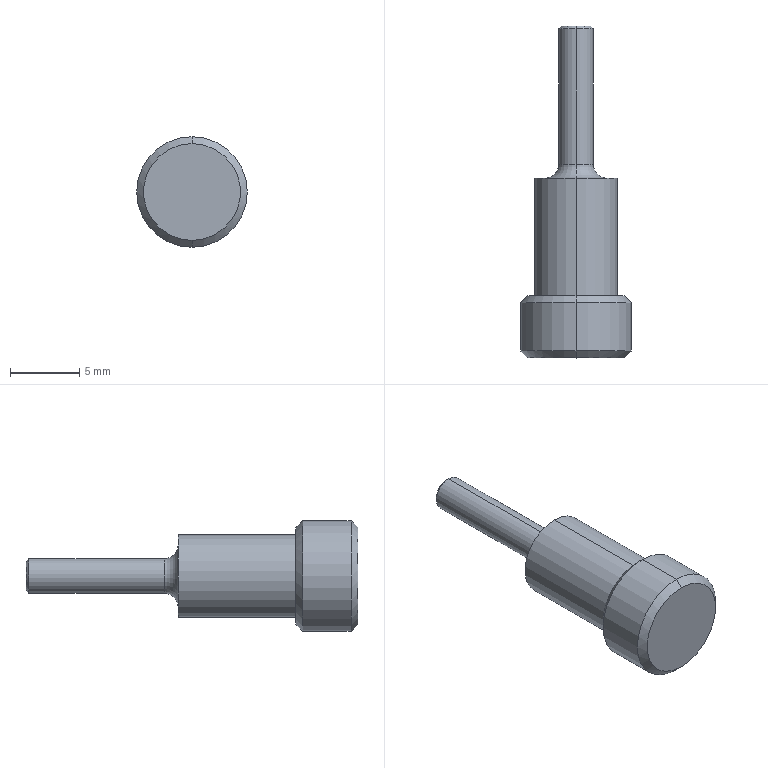Part | SolidWorks | features Chamfer 2, Fillet 1, Revolution 1 | 1 solid | 18 faces | box 8 x 24 x 8 mm | volume 516.339 mm3 | cone 6 | cylinder 6 | plane 4 | torus 2 | commonest cylinder face diameters 2.5 x2 6 x2 8 x2
STEP:
#1=CARTESIAN_POINT('',(0.,24.,1.05));
#2=VERTEX_POINT('',#1);
#3=CARTESIAN_POINT('',(0.,24.,-1.05));
#4=VERTEX_POINT('',#3);
#5=CARTESIAN_POINT('',(0.,24.,0.));
#6=DIRECTION('',(0.,1.,0.));
#7=DIRECTION('',(0.,0.,1.));
#8=AXIS2_PLACEMENT_3D('',#5,#6,#7);
#9=CIRCLE('',#8,1.05);
#10=EDGE_CURVE('',#2,#4,#9,.T.);
#11=ORIENTED_EDGE('',*,*,#10,.F.);
#12=CARTESIAN_POINT('',(0.,23.8,1.25));
#13=VERTEX_POINT('',#12);
#14=CARTESIAN_POINT('',(0.,23.8,1.25));
#15=DIRECTION('',(0.,-0.7071,0.7071));
#16=VECTOR('',#15,1000.);
#17=LINE('',#14,#16);
#18=EDGE_CURVE('',#2,#13,#17,.T.);
#19=ORIENTED_EDGE('',*,*,#18,.T.);
#20=CARTESIAN_POINT('',(0.,23.8,-1.25));
#21=VERTEX_POINT('',#20);
#22=CARTESIAN_POINT('',(0.,23.8,0.));
#23=DIRECTION('',(0.,-1.,0.));
#24=DIRECTION('',(0.,0.,1.));
#25=AXIS2_PLACEMENT_3D('',#22,#23,#24);
#26=CIRCLE('',#25,1.25);
#27=EDGE_CURVE('',#21,#13,#26,.T.);
#28=ORIENTED_EDGE('',*,*,#27,.F.);
#29=CARTESIAN_POINT('',(0.,23.8,-1.25));
#30=DIRECTION('',(0.,-0.7071,-0.7071));
#31=VECTOR('',#30,1000.);
#32=LINE('',#29,#31);
#33=EDGE_CURVE('',#4,#21,#32,.T.);
#34=ORIENTED_EDGE('',*,*,#33,.F.);
#35=EDGE_LOOP('',(#11,#19,#28,#34));
#36=FACE_OUTER_BOUND('',#35,.T.);
#37=CARTESIAN_POINT('',(0.,23.8,0.));
#38=DIRECTION('',(0.,-1.,0.));
#39=DIRECTION('',(0.,0.,-1.));
#40=AXIS2_PLACEMENT_3D('',#37,#38,#39);
#41=CONICAL_SURFACE('',#40,1.25,0.7854);
#42=ADVANCED_FACE('',(#36),#41,.T.);
#43=CARTESIAN_POINT('',(0.,14.,-1.25));
#44=VERTEX_POINT('',#43);
#45=CARTESIAN_POINT('',(0.,14.,1.25));
#46=VERTEX_POINT('',#45);
#47=CARTESIAN_POINT('',(0.,14.,0.));
#48=DIRECTION('',(0.,1.,0.));
#49=DIRECTION('',(0.,0.,1.));
#50=AXIS2_PLACEMENT_3D('',#47,#48,#49);
#51=CIRCLE('',#50,1.25);
#52=EDGE_CURVE('',#44,#46,#51,.T.);
#53=ORIENTED_EDGE('',*,*,#52,.F.);
#54=CARTESIAN_POINT('',(0.,13.,-2.25));
#55=VERTEX_POINT('',#54);
#56=CARTESIAN_POINT('',(0.,14.,-2.25));
#57=DIRECTION('',(1.,0.,0.));
#58=DIRECTION('',(0.,0.,-1.));
#59=AXIS2_PLACEMENT_3D('',#56,#57,#58);
#60=CIRCLE('',#59,1.);
#61=EDGE_CURVE('',#44,#55,#60,.T.);
#62=ORIENTED_EDGE('',*,*,#61,.T.);
#63=CARTESIAN_POINT('',(0.,13.,2.25));
#64=VERTEX_POINT('',#63);
#65=CARTESIAN_POINT('',(0.,13.,0.));
#66=DIRECTION('',(0.,-1.,0.));
#67=DIRECTION('',(0.,0.,1.));
#68=AXIS2_PLACEMENT_3D('',#65,#66,#67);
#69=CIRCLE('',#68,2.25);
#70=EDGE_CURVE('',#64,#55,#69,.T.);
#71=ORIENTED_EDGE('',*,*,#70,.F.);
#72=CARTESIAN_POINT('',(0.,14.,2.25));
#73=DIRECTION('',(-1.,0.,0.));
#74=DIRECTION('',(0.,0.,1.));
#75=AXIS2_PLACEMENT_3D('',#72,#73,#74);
#76=CIRCLE('',#75,1.);
#77=EDGE_CURVE('',#46,#64,#76,.T.);
#78=ORIENTED_EDGE('',*,*,#77,.F.);
#79=EDGE_LOOP('',(#53,#62,#71,#78));
#80=FACE_OUTER_BOUND('',#79,.T.);
#81=CARTESIAN_POINT('',(0.,14.,0.));
#82=DIRECTION('',(0.,1.,0.));
#83=DIRECTION('',(0.,0.,1.));
#84=AXIS2_PLACEMENT_3D('',#81,#82,#83);
#85=TOROIDAL_SURFACE('',#84,2.25,1.);
#86=ADVANCED_FACE('',(#80),#85,.F.);
#87=CARTESIAN_POINT('',(0.,4.5,3.5));
#88=VERTEX_POINT('',#87);
#89=CARTESIAN_POINT('',(0.,4.5,-3.5));
#90=VERTEX_POINT('',#89);
#91=CARTESIAN_POINT('',(0.,4.5,0.));
#92=DIRECTION('',(0.,1.,0.));
#93=DIRECTION('',(0.,0.,1.));
#94=AXIS2_PLACEMENT_3D('',#91,#92,#93);
#95=CIRCLE('',#94,3.5);
#96=EDGE_CURVE('',#88,#90,#95,.T.);
#97=ORIENTED_EDGE('',*,*,#96,.F.);
#98=CARTESIAN_POINT('',(0.,4.,4.));
#99=VERTEX_POINT('',#98);
#100=CARTESIAN_POINT('',(0.,4.,4.));
#101=DIRECTION('',(0.,-0.7071,0.7071));
#102=VECTOR('',#101,1000.);
#103=LINE('',#100,#102);
#104=EDGE_CURVE('',#88,#99,#103,.T.);
#105=ORIENTED_EDGE('',*,*,#104,.T.);
#106=CARTESIAN_POINT('',(0.,4.,-4.));
#107=VERTEX_POINT('',#106);
#108=CARTESIAN_POINT('',(0.,4.,0.));
#109=DIRECTION('',(0.,-1.,0.));
#110=DIRECTION('',(0.,0.,1.));
#111=AXIS2_PLACEMENT_3D('',#108,#109,#110);
#112=CIRCLE('',#111,4.);
#113=EDGE_CURVE('',#107,#99,#112,.T.);
#114=ORIENTED_EDGE('',*,*,#113,.F.);
#115=CARTESIAN_POINT('',(0.,4.,-4.));
#116=DIRECTION('',(0.,-0.7071,-0.7071));
#117=VECTOR('',#116,1000.);
#118=LINE('',#115,#117);
#119=EDGE_CURVE('',#90,#107,#118,.T.);
#120=ORIENTED_EDGE('',*,*,#119,.F.);
#121=EDGE_LOOP('',(#97,#105,#114,#120));
#122=FACE_OUTER_BOUND('',#121,.T.);
#123=CARTESIAN_POINT('',(0.,4.,0.));
#124=DIRECTION('',(0.,-1.,0.));
#125=DIRECTION('',(0.,0.,-1.));
#126=AXIS2_PLACEMENT_3D('',#123,#124,#125);
#127=CONICAL_SURFACE('',#126,4.,0.7854);
#128=ADVANCED_FACE('',(#122),#127,.T.);
#129=CARTESIAN_POINT('',(0.,0.,-3.5));
#130=VERTEX_POINT('',#129);
#131=CARTESIAN_POINT('',(0.,0.,3.5));
#132=VERTEX_POINT('',#131);
#133=CARTESIAN_POINT('',(0.,0.,0.));
#134=DIRECTION('',(0.,-1.,0.));
#135=DIRECTION('',(0.,0.,-1.));
#136=AXIS2_PLACEMENT_3D('',#133,#134,#135);
#137=CIRCLE('',#136,3.5);
#138=EDGE_CURVE('',#130,#132,#137,.T.);
#139=ORIENTED_EDGE('',*,*,#138,.F.);
#140=CARTESIAN_POINT('',(0.,0.5,-4.));
#141=VERTEX_POINT('',#140);
#142=CARTESIAN_POINT('',(0.,0.,-3.5));
#143=DIRECTION('',(0.,0.7071,-0.7071));
#144=VECTOR('',#143,1000.);
#145=LINE('',#142,#144);
#146=EDGE_CURVE('',#130,#141,#145,.T.);
#147=ORIENTED_EDGE('',*,*,#146,.T.);
#148=CARTESIAN_POINT('',(0.,0.5,4.));
#149=VERTEX_POINT('',#148);
#150=CARTESIAN_POINT('',(0.,0.5,0.));
#151=DIRECTION('',(0.,1.,0.));
#152=DIRECTION('',(0.,0.,-1.));
#153=AXIS2_PLACEMENT_3D('',#150,#151,#152);
#154=CIRCLE('',#153,4.);
#155=EDGE_CURVE('',#149,#141,#154,.T.);
#156=ORIENTED_EDGE('',*,*,#155,.F.);
#157=CARTESIAN_POINT('',(0.,0.,3.5));
#158=DIRECTION('',(0.,0.7071,0.7071));
#159=VECTOR('',#158,1000.);
#160=LINE('',#157,#159);
#161=EDGE_CURVE('',#132,#149,#160,.T.);
#162=ORIENTED_EDGE('',*,*,#161,.F.);
#163=EDGE_LOOP('',(#139,#147,#156,#162));
#164=FACE_OUTER_BOUND('',#163,.T.);
#165=CARTESIAN_POINT('',(0.,0.,0.));
#166=DIRECTION('',(0.,1.,0.));
#167=DIRECTION('',(0.,0.,1.));
#168=AXIS2_PLACEMENT_3D('',#165,#166,#167);
#169=CONICAL_SURFACE('',#168,3.5,0.7854);
#170=ADVANCED_FACE('',(#164),#169,.T.);
#171=ORIENTED_EDGE('',*,*,#113,.T.);
#172=CARTESIAN_POINT('',(0.,-0.5244,4.));
#173=DIRECTION('',(0.,-1.,0.));
#174=VECTOR('',#173,1000.);
#175=LINE('',#172,#174);
#176=EDGE_CURVE('',#99,#149,#175,.T.);
#177=ORIENTED_EDGE('',*,*,#176,.T.);
#178=ORIENTED_EDGE('',*,*,#155,.T.);
#179=CARTESIAN_POINT('',(0.,-0.5244,-4.));
#180=DIRECTION('',(0.,-1.,0.));
#181=VECTOR('',#180,1000.);
#182=LINE('',#179,#181);
#183=EDGE_CURVE('',#107,#141,#182,.T.);
#184=ORIENTED_EDGE('',*,*,#183,.F.);
#185=EDGE_LOOP('',(#171,#177,#178,#184));
#186=FACE_OUTER_BOUND('',#185,.T.);
#187=CARTESIAN_POINT('',(0.,-0.5244,0.));
#188=DIRECTION('',(0.,-1.,0.));
#189=DIRECTION('',(0.,0.,-1.));
#190=AXIS2_PLACEMENT_3D('',#187,#188,#189);
#191=CYLINDRICAL_SURFACE('',#190,4.);
#192=ADVANCED_FACE('',(#186),#191,.T.);
#193=CARTESIAN_POINT('',(0.,13.,-3.));
#194=VERTEX_POINT('',#193);
#195=CARTESIAN_POINT('',(0.,13.,3.));
#196=VERTEX_POINT('',#195);
#197=CARTESIAN_POINT('',(0.,13.,0.));
#198=DIRECTION('',(0.,-1.,0.));
#199=DIRECTION('',(0.,0.,-1.));
#200=AXIS2_PLACEMENT_3D('',#197,#198,#199);
#201=CIRCLE('',#200,3.);
#202=EDGE_CURVE('',#194,#196,#201,.T.);
#203=ORIENTED_EDGE('',*,*,#202,.T.);
#204=CARTESIAN_POINT('',(0.,4.5,3.));
#205=VERTEX_POINT('',#204);
#206=CARTESIAN_POINT('',(0.,-0.5244,3.));
#207=DIRECTION('',(0.,-1.,0.));
#208=VECTOR('',#207,1000.);
#209=LINE('',#206,#208);
#210=EDGE_CURVE('',#196,#205,#209,.T.);
#211=ORIENTED_EDGE('',*,*,#210,.T.);
#212=CARTESIAN_POINT('',(0.,4.5,-3.));
#213=VERTEX_POINT('',#212);
#214=CARTESIAN_POINT('',(0.,4.5,0.));
#215=DIRECTION('',(0.,-1.,0.));
#216=DIRECTION('',(0.,0.,-1.));
#217=AXIS2_PLACEMENT_3D('',#214,#215,#216);
#218=CIRCLE('',#217,3.);
#219=EDGE_CURVE('',#213,#205,#218,.T.);
#220=ORIENTED_EDGE('',*,*,#219,.F.);
#221=CARTESIAN_POINT('',(0.,-0.5244,-3.));
#222=DIRECTION('',(0.,-1.,0.));
#223=VECTOR('',#222,1000.);
#224=LINE('',#221,#223);
#225=EDGE_CURVE('',#194,#213,#224,.T.);
#226=ORIENTED_EDGE('',*,*,#225,.F.);
#227=EDGE_LOOP('',(#203,#211,#220,#226));
#228=FACE_OUTER_BOUND('',#227,.T.);
#229=CARTESIAN_POINT('',(0.,-0.5244,0.));
#230=DIRECTION('',(0.,-1.,0.));
#231=DIRECTION('',(0.,0.,-1.));
#232=AXIS2_PLACEMENT_3D('',#229,#230,#231);
#233=CYLINDRICAL_SURFACE('',#232,3.);
#234=ADVANCED_FACE('',(#228),#233,.T.);
#235=ORIENTED_EDGE('',*,*,#27,.T.);
#236=CARTESIAN_POINT('',(0.,-0.5244,1.25));
#237=DIRECTION('',(0.,-1.,0.));
#238=VECTOR('',#237,1000.);
#239=LINE('',#236,#238);
#240=EDGE_CURVE('',#13,#46,#239,.T.);
#241=ORIENTED_EDGE('',*,*,#240,.T.);
#242=CARTESIAN_POINT('',(0.,14.,0.));
#243=DIRECTION('',(0.,1.,0.));
#244=DIRECTION('',(0.,0.,1.));
#245=AXIS2_PLACEMENT_3D('',#242,#243,#244);
#246=CIRCLE('',#245,1.25);
#247=EDGE_CURVE('',#46,#44,#246,.T.);
#248=ORIENTED_EDGE('',*,*,#247,.T.);
#249=CARTESIAN_POINT('',(0.,-0.5244,-1.25));
#250=DIRECTION('',(0.,-1.,0.));
#251=VECTOR('',#250,1000.);
#252=LINE('',#249,#251);
#253=EDGE_CURVE('',#21,#44,#252,.T.);
#254=ORIENTED_EDGE('',*,*,#253,.F.);
#255=EDGE_LOOP('',(#235,#241,#248,#254));
#256=FACE_OUTER_BOUND('',#255,.T.);
#257=CARTESIAN_POINT('',(0.,-0.5244,0.));
#258=DIRECTION('',(0.,-1.,0.));
#259=DIRECTION('',(0.,0.,-1.));
#260=AXIS2_PLACEMENT_3D('',#257,#258,#259);
#261=CYLINDRICAL_SURFACE('',#260,1.25);
#262=ADVANCED_FACE('',(#256),#261,.T.);
#263=CARTESIAN_POINT('',(0.,24.,0.));
#264=DIRECTION('',(0.,1.,0.));
#265=DIRECTION('',(0.,0.,1.));
#266=AXIS2_PLACEMENT_3D('',#263,#264,#265);
#267=CIRCLE('',#266,1.05);
#268=EDGE_CURVE('',#4,#2,#267,.T.);
#269=ORIENTED_EDGE('',*,*,#268,.T.);
#270=ORIENTED_EDGE('',*,*,#10,.T.);
#271=EDGE_LOOP('',(#269,#270));
#272=FACE_OUTER_BOUND('',#271,.T.);
#273=CARTESIAN_POINT('',(0.,24.,0.));
#274=DIRECTION('',(0.,1.,0.));
#275=DIRECTION('',(0.,0.,1.));
#276=AXIS2_PLACEMENT_3D('',#273,#274,#275);
#277=PLANE('',#276);
#278=ADVANCED_FACE('',(#272),#277,.T.);
#279=ORIENTED_EDGE('',*,*,#240,.F.);
#280=CARTESIAN_POINT('',(0.,23.8,0.));
#281=DIRECTION('',(0.,-1.,0.));
#282=DIRECTION('',(0.,0.,1.));
#283=AXIS2_PLACEMENT_3D('',#280,#281,#282);
#284=CIRCLE('',#283,1.25);
#285=EDGE_CURVE('',#13,#21,#284,.T.);
#286=ORIENTED_EDGE('',*,*,#285,.T.);
#287=ORIENTED_EDGE('',*,*,#253,.T.);
#288=ORIENTED_EDGE('',*,*,#52,.T.);
#289=EDGE_LOOP('',(#279,#286,#287,#288));
#290=FACE_OUTER_BOUND('',#289,.T.);
#291=CARTESIAN_POINT('',(0.,-0.5244,0.));
#292=DIRECTION('',(0.,-1.,0.));
#293=DIRECTION('',(0.,0.,-1.));
#294=AXIS2_PLACEMENT_3D('',#291,#292,#293);
#295=CYLINDRICAL_SURFACE('',#294,1.25);
#296=ADVANCED_FACE('',(#290),#295,.T.);
#297=ORIENTED_EDGE('',*,*,#70,.T.);
#298=CARTESIAN_POINT('',(0.,13.,0.));
#299=DIRECTION('',(0.,-1.,0.));
#300=DIRECTION('',(0.,0.,1.));
#301=AXIS2_PLACEMENT_3D('',#298,#299,#300);
#302=CIRCLE('',#301,2.25);
#303=EDGE_CURVE('',#55,#64,#302,.T.);
#304=ORIENTED_EDGE('',*,*,#303,.T.);
#305=EDGE_LOOP('',(#297,#304));
#306=FACE_BOUND('',#305,.T.);
#307=ORIENTED_EDGE('',*,*,#202,.F.);
#308=CARTESIAN_POINT('',(0.,13.,0.));
#309=DIRECTION('',(0.,-1.,0.));
#310=DIRECTION('',(0.,0.,-1.));
#311=AXIS2_PLACEMENT_3D('',#308,#309,#310);
#312=CIRCLE('',#311,3.);
#313=EDGE_CURVE('',#196,#194,#312,.T.);
#314=ORIENTED_EDGE('',*,*,#313,.F.);
#315=EDGE_LOOP('',(#307,#314));
#316=FACE_OUTER_BOUND('',#315,.T.);
#317=CARTESIAN_POINT('',(1.25,13.,0.));
#318=DIRECTION('',(0.,1.,0.));
#319=DIRECTION('',(0.,0.,1.));
#320=AXIS2_PLACEMENT_3D('',#317,#318,#319);
#321=PLANE('',#320);
#322=ADVANCED_FACE('',(#306,#316),#321,.T.);
#323=ORIENTED_EDGE('',*,*,#210,.F.);
#324=ORIENTED_EDGE('',*,*,#313,.T.);
#325=ORIENTED_EDGE('',*,*,#225,.T.);
#326=CARTESIAN_POINT('',(0.,4.5,0.));
#327=DIRECTION('',(0.,-1.,0.));
#328=DIRECTION('',(0.,0.,-1.));
#329=AXIS2_PLACEMENT_3D('',#326,#327,#328);
#330=CIRCLE('',#329,3.);
#331=EDGE_CURVE('',#205,#213,#330,.T.);
#332=ORIENTED_EDGE('',*,*,#331,.F.);
#333=EDGE_LOOP('',(#323,#324,#325,#332));
#334=FACE_OUTER_BOUND('',#333,.T.);
#335=CARTESIAN_POINT('',(0.,-0.5244,0.));
#336=DIRECTION('',(0.,-1.,0.));
#337=DIRECTION('',(0.,0.,-1.));
#338=AXIS2_PLACEMENT_3D('',#335,#336,#337);
#339=CYLINDRICAL_SURFACE('',#338,3.);
#340=ADVANCED_FACE('',(#334),#339,.T.);
#341=CARTESIAN_POINT('',(0.,4.5,0.));
#342=DIRECTION('',(0.,1.,0.));
#343=DIRECTION('',(0.,0.,1.));
#344=AXIS2_PLACEMENT_3D('',#341,#342,#343);
#345=CIRCLE('',#344,3.5);
#346=EDGE_CURVE('',#90,#88,#345,.T.);
#347=ORIENTED_EDGE('',*,*,#346,.T.);
#348=ORIENTED_EDGE('',*,*,#96,.T.);
#349=EDGE_LOOP('',(#347,#348));
#350=FACE_OUTER_BOUND('',#349,.T.);
#351=ORIENTED_EDGE('',*,*,#219,.T.);
#352=ORIENTED_EDGE('',*,*,#331,.T.);
#353=EDGE_LOOP('',(#351,#352));
#354=FACE_BOUND('',#353,.T.);
#355=CARTESIAN_POINT('',(3.,4.5,0.));
#356=DIRECTION('',(0.,1.,0.));
#357=DIRECTION('',(0.,0.,1.));
#358=AXIS2_PLACEMENT_3D('',#355,#356,#357);
#359=PLANE('',#358);
#360=ADVANCED_FACE('',(#350,#354),#359,.T.);
#361=ORIENTED_EDGE('',*,*,#176,.F.);
#362=CARTESIAN_POINT('',(0.,4.,0.));
#363=DIRECTION('',(0.,-1.,0.));
#364=DIRECTION('',(0.,0.,1.));
#365=AXIS2_PLACEMENT_3D('',#362,#363,#364);
#366=CIRCLE('',#365,4.);
#367=EDGE_CURVE('',#99,#107,#366,.T.);
#368=ORIENTED_EDGE('',*,*,#367,.T.);
#369=ORIENTED_EDGE('',*,*,#183,.T.);
#370=CARTESIAN_POINT('',(0.,0.5,0.));
#371=DIRECTION('',(0.,1.,0.));
#372=DIRECTION('',(0.,0.,-1.));
#373=AXIS2_PLACEMENT_3D('',#370,#371,#372);
#374=CIRCLE('',#373,4.);
#375=EDGE_CURVE('',#141,#149,#374,.T.);
#376=ORIENTED_EDGE('',*,*,#375,.T.);
#377=EDGE_LOOP('',(#361,#368,#369,#376));
#378=FACE_OUTER_BOUND('',#377,.T.);
#379=CARTESIAN_POINT('',(0.,-0.5244,0.));
#380=DIRECTION('',(0.,-1.,0.));
#381=DIRECTION('',(0.,0.,-1.));
#382=AXIS2_PLACEMENT_3D('',#379,#380,#381);
#383=CYLINDRICAL_SURFACE('',#382,4.);
#384=ADVANCED_FACE('',(#378),#383,.T.);
#385=CARTESIAN_POINT('',(0.,0.,0.));
#386=DIRECTION('',(0.,-1.,0.));
#387=DIRECTION('',(0.,0.,-1.));
#388=AXIS2_PLACEMENT_3D('',#385,#386,#387);
#389=CIRCLE('',#388,3.5);
#390=EDGE_CURVE('',#132,#130,#389,.T.);
#391=ORIENTED_EDGE('',*,*,#390,.T.);
#392=ORIENTED_EDGE('',*,*,#138,.T.);
#393=EDGE_LOOP('',(#391,#392));
#394=FACE_OUTER_BOUND('',#393,.T.);
#395=CARTESIAN_POINT('',(0.,0.,0.));
#396=DIRECTION('',(0.,-1.,0.));
#397=DIRECTION('',(0.,0.,-1.));
#398=AXIS2_PLACEMENT_3D('',#395,#396,#397);
#399=PLANE('',#398);
#400=ADVANCED_FACE('',(#394),#399,.T.);
#401=ORIENTED_EDGE('',*,*,#146,.F.);
#402=ORIENTED_EDGE('',*,*,#390,.F.);
#403=ORIENTED_EDGE('',*,*,#161,.T.);
#404=ORIENTED_EDGE('',*,*,#375,.F.);
#405=EDGE_LOOP('',(#401,#402,#403,#404));
#406=FACE_OUTER_BOUND('',#405,.T.);
#407=CARTESIAN_POINT('',(0.,0.,0.));
#408=DIRECTION('',(0.,1.,0.));
#409=DIRECTION('',(0.,0.,1.));
#410=AXIS2_PLACEMENT_3D('',#407,#408,#409);
#411=CONICAL_SURFACE('',#410,3.5,0.7854);
#412=ADVANCED_FACE('',(#406),#411,.T.);
#413=ORIENTED_EDGE('',*,*,#104,.F.);
#414=ORIENTED_EDGE('',*,*,#346,.F.);
#415=ORIENTED_EDGE('',*,*,#119,.T.);
#416=ORIENTED_EDGE('',*,*,#367,.F.);
#417=EDGE_LOOP('',(#413,#414,#415,#416));
#418=FACE_OUTER_BOUND('',#417,.T.);
#419=CARTESIAN_POINT('',(0.,4.,0.));
#420=DIRECTION('',(0.,-1.,0.));
#421=DIRECTION('',(0.,0.,-1.));
#422=AXIS2_PLACEMENT_3D('',#419,#420,#421);
#423=CONICAL_SURFACE('',#422,4.,0.7854);
#424=ADVANCED_FACE('',(#418),#423,.T.);
#425=ORIENTED_EDGE('',*,*,#61,.F.);
#426=ORIENTED_EDGE('',*,*,#247,.F.);
#427=ORIENTED_EDGE('',*,*,#77,.T.);
#428=ORIENTED_EDGE('',*,*,#303,.F.);
#429=EDGE_LOOP('',(#425,#426,#427,#428));
#430=FACE_OUTER_BOUND('',#429,.T.);
#431=CARTESIAN_POINT('',(0.,14.,0.));
#432=DIRECTION('',(0.,1.,0.));
#433=DIRECTION('',(0.,0.,1.));
#434=AXIS2_PLACEMENT_3D('',#431,#432,#433);
#435=TOROIDAL_SURFACE('',#434,2.25,1.);
#436=ADVANCED_FACE('',(#430),#435,.F.);
#437=ORIENTED_EDGE('',*,*,#18,.F.);
#438=ORIENTED_EDGE('',*,*,#268,.F.);
#439=ORIENTED_EDGE('',*,*,#33,.T.);
#440=ORIENTED_EDGE('',*,*,#285,.F.);
#441=EDGE_LOOP('',(#437,#438,#439,#440));
#442=FACE_OUTER_BOUND('',#441,.T.);
#443=CARTESIAN_POINT('',(0.,23.8,0.));
#444=DIRECTION('',(0.,-1.,0.));
#445=DIRECTION('',(0.,0.,-1.));
#446=AXIS2_PLACEMENT_3D('',#443,#444,#445);
#447=CONICAL_SURFACE('',#446,1.25,0.7854);
#448=ADVANCED_FACE('',(#442),#447,.T.);
#449=CLOSED_SHELL('',(#42,#86,#128,#170,#192,#234,#262,#278,#296,#322,#340,#360,#384,#400,#412,#424,#436,#448));
#450=MANIFOLD_SOLID_BREP('',#449);
#451=CARTESIAN_POINT('',(0.,0.,0.));
#452=DIRECTION('',(0.,0.,1.));
#453=DIRECTION('',(1.,0.,0.));
#454=AXIS2_PLACEMENT_3D('',#451,#452,#453);
#455=(LENGTH_UNIT()NAMED_UNIT(*)SI_UNIT(.MILLI.,.METRE.));
#456=UNCERTAINTY_MEASURE_WITH_UNIT(LENGTH_MEASURE(0.00001),#455,'','');
#457=(NAMED_UNIT(*)PLANE_ANGLE_UNIT()SI_UNIT($,.RADIAN.));
#458=(NAMED_UNIT(*)SI_UNIT($,.STERADIAN.)SOLID_ANGLE_UNIT());
#459=(GEOMETRIC_REPRESENTATION_CONTEXT(3)GLOBAL_UNCERTAINTY_ASSIGNED_CONTEXT((#456))GLOBAL_UNIT_ASSIGNED_CONTEXT((#455,#457,#458))REPRESENTATION_CONTEXT('',''));
#460=ADVANCED_BREP_SHAPE_REPRESENTATION('',(#450,#454),#459);